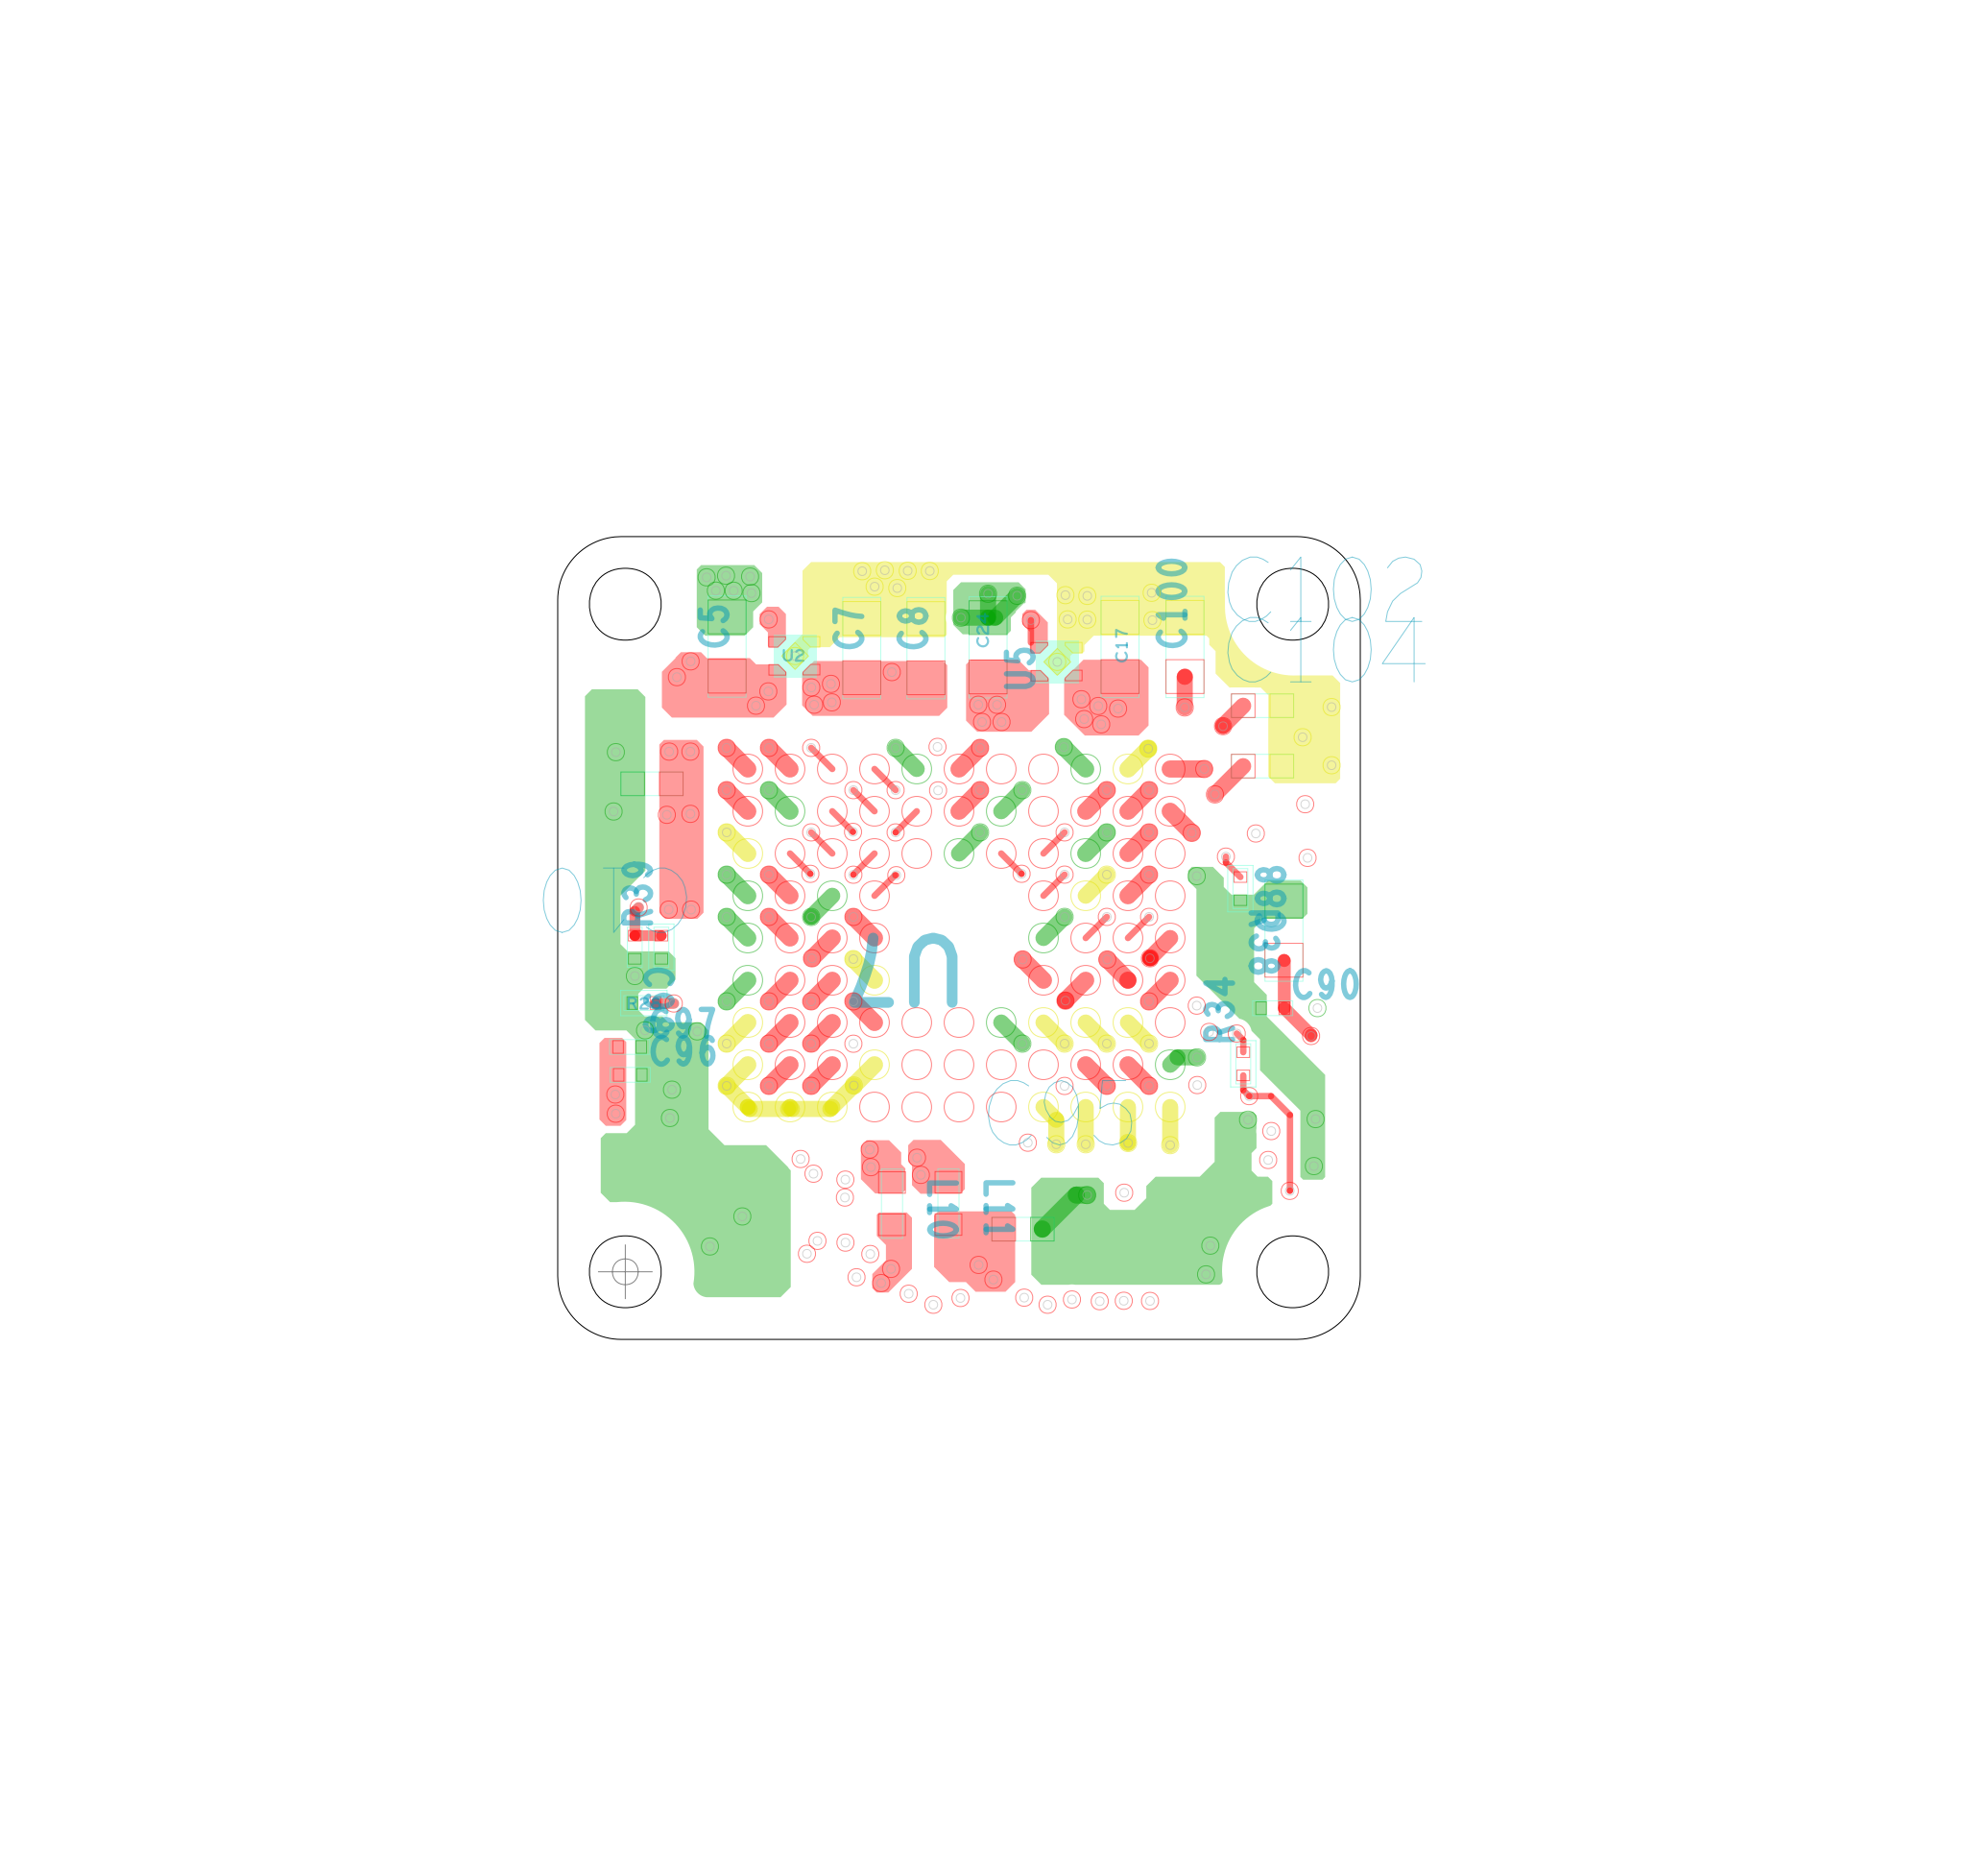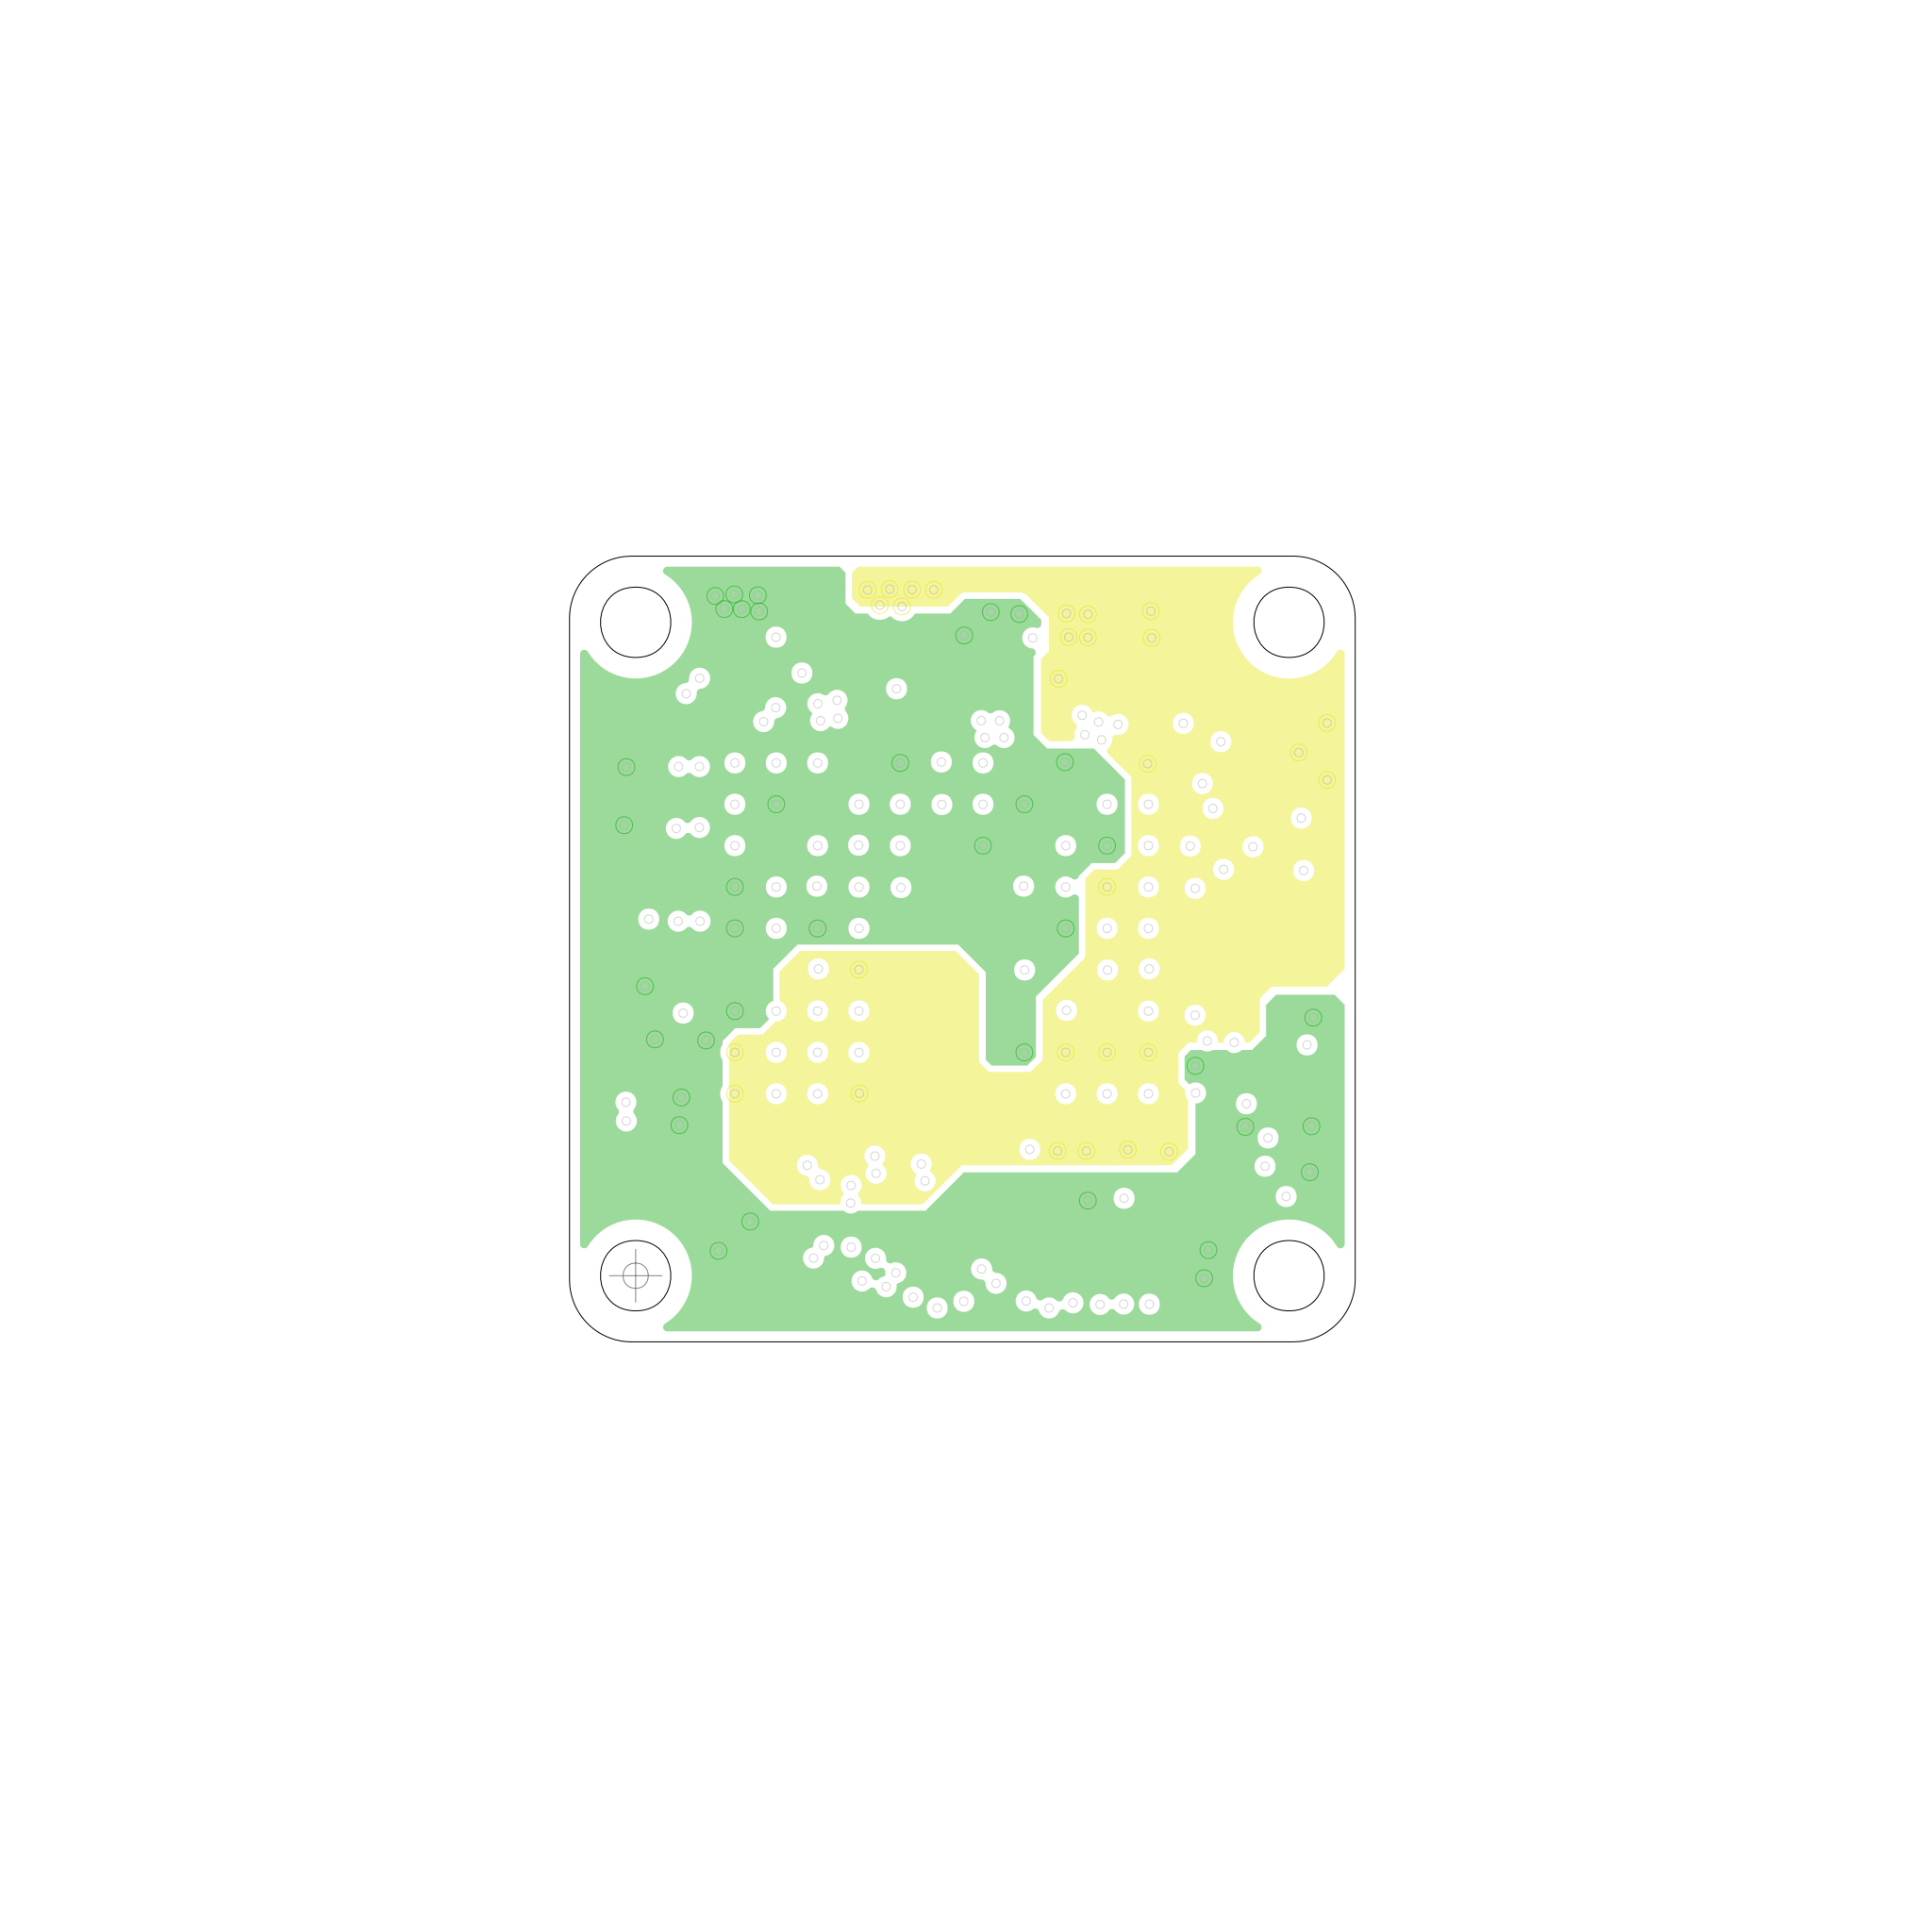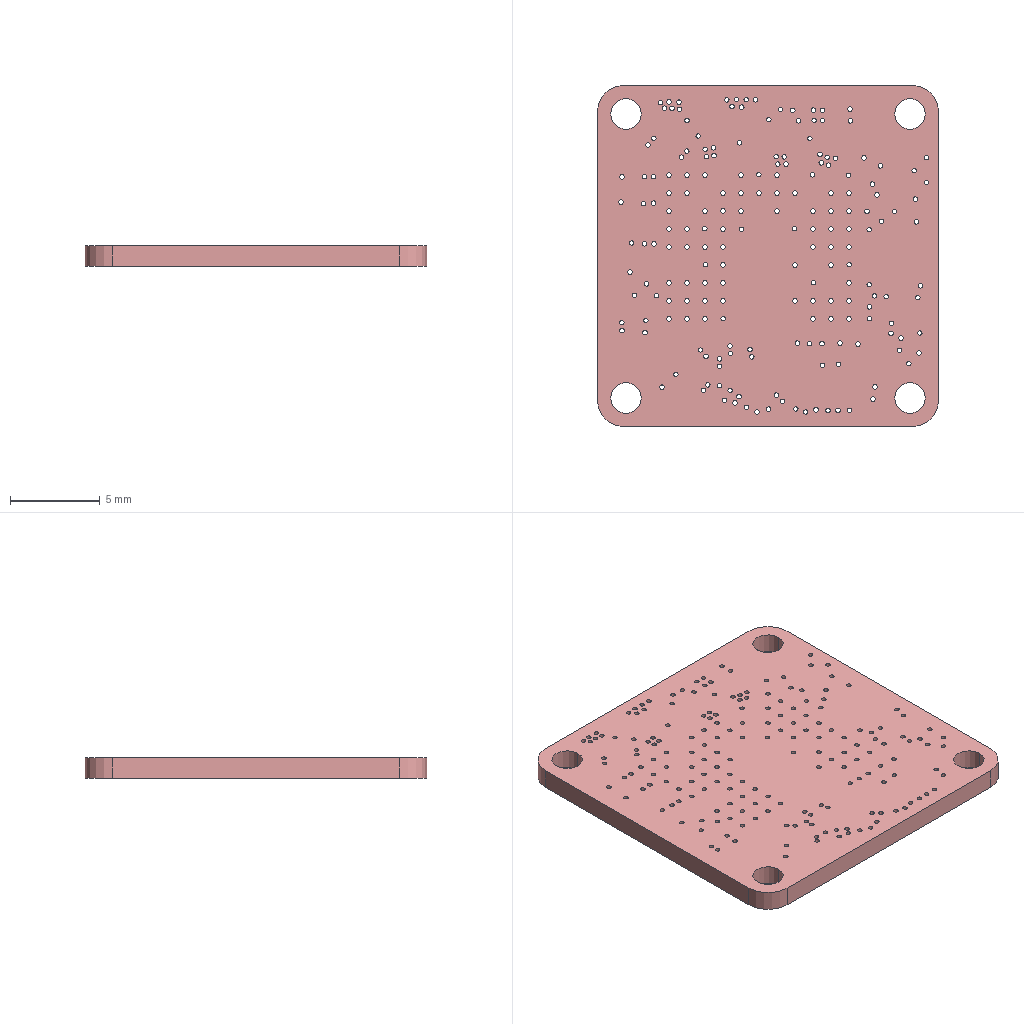Circuit board layout | Cadence Allegro | box 19 x 19 x 1.1 mm
Layer stack:
# Cadence Allegro layer stack of  (unit mm; from the constraint file cross-section; dielectric type: 0 not recorded (Allegro does not mark core vs prepreg), 3 surface material)
index,name,kind,layer,copper_thickness_mm,dielectric_type,dielectric_thickness_mm,dielectric_material,dielectric_constant
0,Top Surface,other,,,,,,
1,TOP,copper,TOP,0.0305,,,,
2,Dielectric1,dielectric,,,0,0.2032,FR-4,4.5
3,GND02,copper,GND02,0.0305,,,,
4,Dielectric2,dielectric,,,0,0.2032,FR-4,4.5
5,SIG03,copper,SIG03,0.0305,,,,
6,Dielectric3,dielectric,,,0,0.2032,FR-4,4.5
7,PWR04,copper,PWR04,0.0305,,,,
8,Dielectric4,dielectric,,,0,0.2032,FR-4,4.5
9,POWER5,copper,POWER5,0.0305,,,,
10,Dielectric5,dielectric,,,0,0.2032,FR-4,4.5
11,BOTTOM,copper,BOTTOM,0.0305,,,,
12,Bottom Surface,other,,,,,,
# drill layer pairs: low layer,high layer
drill_pair,TOP,BOTTOM
Part placement:
REFDES,COMP_VALUE,SYM_NAME,SYM_X,SYM_Y,SYM_ROTATE,SYM_MIRROR
C5,22uF,C0603,94.89,582.62,90.000,NO
C7,22uF,C0603,220.41,581.18,90.000,NO
C8,10uF,C0603,280.21,581.08,90.000,NO
C9,22uF,C0603,19.28,513.11,0.000,YES
C10,10uF,C0402,24.68,454.69,180.000,NO
C11,0.1uF,C0201,153.59,461.18,90.000,YES
C17,22uF,C0603,461.12,582.21,90.000,NO
C18,10uF,C0603,461.58,582.19,270.000,YES
C19,4.7uF,C0402,129.21,412.53,135.000,YES
C20,0.1uF,C0201,114.20,232.60,0.000,YES
C21,0.1uF,C0201,114.42,193.91,0.000,YES
C24,22uF,C0603,338.10,581.90,90.000,NO
C25,22uF,C0603,17.11,198.08,180.000,YES
C28,0.1uF,C0201,389.89,260.78,90.000,YES
C29,0.1uF,C0201,428.89,242.68,90.000,YES
C30,0.1uF,C0201,191.87,270.53,225.000,YES
C80,22uF,C0603,18.79,454.24,0.000,YES
C83,0.1uF,C0201,113.59,310.80,0.000,YES
C84,0.1uF,C0201,194.09,349.40,0.000,YES
C85,4.7uF,C0402,220.47,591.01,270.000,YES
C86,2.2uF,C0201,600.20,192.90,90.000,YES
C87,0.1uF,C0201,348.90,208.99,270.000,YES
C88,22uF,C0603,613.90,317.90,90.000,NO
C89,0.1uF,C0201,509.50,218.20,90.000,YES
C90,2.2uF,C0201,603.40,245.60,0.000,NO
C91,4.7uF,C0402,331.27,574.61,270.000,YES
C92,0.1uF,C0201,364.60,568.20,270.000,YES
C93,4.7uF,C0402,94.47,590.71,270.000,YES
C94,0.1uF,C0201,129.40,572.90,270.000,YES
C95,4.7uF,C0402,370.90,39.70,0.000,NO
C96,2.2uF,C0201,4.60,183.50,0.000,NO
C97,2.2uF,C0201,4.10,209.50,0.000,NO
C98,2.2uF,C0201,8.80,302.39,270.000,NO
C99,22uF,C0603,604.00,527.70,180.000,YES
C100,22uF,C0603,521.66,582.21,90.000,NO
C101,22uF,C0603,603.81,469.66,180.000,YES
C102,4.7uF,C0402,594.11,527.47,0.000,NO
C103,4.7uF,C0402,521.27,573.31,270.000,YES
C104,4.7uF,C0402,594.11,471.17,0.000,NO
J2,MIPI_OUT,J30-0_6MM,122.05,143.31,180.000,YES
L7,4.7uH,IND2-2R0X1R6,-13.58,383.84,180.000,YES
L10,0R,R0402,248.60,63.50,270.000,NO
L11,0R,R0402,301.20,63.70,270.000,NO
L12,NC,R0402,279.90,553.80,90.000,YES
L13,0R,R0402,156.20,635.90,180.000,YES
R27,100K,R0201,63.41,260.82,270.000,YES
R28,115K,R0201,17.32,250.41,0.000,NO
R33,0R,R0201,624.30,193.30,90.000,YES
R34,NC,R0201,576.00,193.80,90.000,NO
R35,1K,R0201,373.51,418.43,180.000,YES
R36,1K,R0201,373.71,392.33,180.000,YES
R37,2K,R0201,553.10,193.90,90.000,YES
R38,0R,R0201,573.30,357.00,270.000,NO
R39,NC,R0201,33.60,302.41,90.000,NO
R40,NC,R0201,609.30,411.10,270.000,YES
R41,NC,R0201,633.70,410.90,270.000,YES
R42,0R,R0201,576.00,193.40,270.000,YES
TP4,TestPoint,TP_0R50,114.82,4.21,0.000,YES
TP6,TestPoint,TP_0R50,155.89,2.37,0.000,YES
TP7,TestPoint,TP_0R50,197.19,-0.23,0.000,YES
TP8,TestPoint,TP_0R50,241.30,204.40,0.000,YES
TP9,TestPoint,TP_0R50,279.40,204.00,0.000,YES
TP10,TestPoint,TP_0R50,78.89,3.97,0.000,YES
U2,SGM2036-1.8V UTDFN,UTDFN_1X1-4L,158.26,573.78,90.000,NO
U5,SGM2036-2.8V UTDFN,UTDFN_1X1-4L,402.63,568.31,90.000,NO
U7,IMX600,SENSOR,311.02,311.02,180.000,NO
U9,MP1601,SOT563_1R5X1R2,28.60,253.90,0.000,YES
U13,MPU6600 QFN24,MCU_QFN20_S120,649.14,343.35,0.000,YES
U14,CZ,0201_3,464.60,4.50,0.000,YES
U15,CZ,0201_3,393.60,5.10,0.000,YES
U16,CZ,0201_3,287.10,5.20,180.000,YES
Pad and via stacks:
# Allegro (Cadence) via spans and padstacks; design units: ("mils" 2 100)
# via spans: padstack,start_layer,end_layer,net_example,count
VIA-8X16,ETCH/TOP,ETCH/BOTTOM,GND,191
# Allegro padstack definitions: name,start_layer,end_layer,drill,plating,holeType,type
S_R0R80X0R90,"ETCH/TOP","ETCH/TOP",0.0,"PLATED","none","smd"
S_R0R25X0R30,"ETCH/TOP","ETCH/TOP",0.0,"NON_PLATED","none","smd"
SMD22_22,"ETCH/TOP","ETCH/TOP",0.0,"PLATED","none","smd"
SMD0D25X0D65,"ETCH/TOP","ETCH/TOP",0.0,"PLATED","none","smd"
SMD0R775_1R0,"ETCH/TOP","ETCH/TOP",0.0,"PLATED","none","smd"
SMD0R7SQ,"ETCH/TOP","ETCH/TOP",0.0,"PLATED","none","smd"
S_R0R70X2R00,"ETCH/TOP","ETCH/TOP",0.0,"NON_PLATED","none","smd"
SMD19_20PSH_L,"ETCH/TOP","ETCH/TOP",0.0,"PLATED","none","smd"
SMD19_20PSH_R,"ETCH/TOP","ETCH/TOP",0.0,"PLATED","none","smd"
SMD_BOTTOM_R350X300P0S40,"ETCH/TOP","ETCH/TOP",0.0,"PLATED","none","smd"
S_C0R50,"ETCH/TOP","ETCH/TOP",0.0,"NON_PLATED","none","smd"
SMD40REC20,"ETCH/TOP","ETCH/TOP",0.0,"PLATED","none","smd"
S_S0R45,"ETCH/TOP","ETCH/TOP",0.0,"NON_PLATED","none","smd"
UTDFN_1,"ETCH/TOP","ETCH/TOP",0.0,"PLATED","none","smd"
UTDFN_2,"ETCH/TOP","ETCH/TOP",0.0,"PLATED","none","smd"
SMD5-0,"ETCH/TOP","ETCH/TOP",0.0,"NON_PLATED","none","smd"
SMD0-8_0-15,"ETCH/TOP","ETCH/TOP",0.0,"NON_PLATED","none","smd"
SMD_C118P0S40,"ETCH/TOP","ETCH/TOP",0.0,"PLATED","none","smd"
SMD_R12X27,"ETCH/TOP","ETCH/TOP",0.0,"PLATED","none","smd"
SMD_R118X236P0S40,"ETCH/TOP","ETCH/TOP",0.0,"PLATED","none","smd"
SMD_0D8X0D9,"ETCH/TOP","ETCH/TOP",0.0,"PLATED","none","smd"
SMD5-0-1,"ETCH/TOP","ETCH/TOP",0.0,"NON_PLATED","none","smd"
SMD59_35,"ETCH/TOP","ETCH/TOP",0.0,"PLATED","none","smd"
P_C0R40_C0R65,"ETCH/TOP","ETCH/BOTTOM",15.7,"PLATED","circle_drill","through"
VIA,"ETCH/TOP","ETCH/BOTTOM",13.0,"PLATED","circle_drill","through"
VIA_FORPCB_8X16,"ETCH/TOP","ETCH/BOTTOM",8.0,"PLATED","circle_drill","through"
PTH_C1063D984S50,"ETCH/TOP","ETCH/BOTTOM",74.8,"PLATED","circle_drill","through"
HOLE2-3_5,"ETCH/TOP","ETCH/BOTTOM",82.7,"PLATED","circle_drill","through"
VIA_FORPCB_10X18,"ETCH/TOP","ETCH/BOTTOM",10.0,"PLATED","circle_drill","through"
SMD0R45_CIR,"ETCH/TOP","ETCH/TOP",0.0,"PLATED","none","smd"
SMD1R1_SQ,"ETCH/TOP","ETCH/TOP",0.0,"PLATED","none","smd"
S_C0R50-1,"ETCH/TOP","ETCH/TOP",0.0,"NON_PLATED","none","smd"
S_C0R50-2,"ETCH/TOP","ETCH/TOP",0.0,"NON_PLATED","none","smd"
SMD1R0_CIR,"ETCH/TOP","ETCH/TOP",0.0,"PLATED","none","smd"
SMD1R6X0R7,"ETCH/TOP","ETCH/TOP",0.0,"PLATED","none","smd"
SMD0-25_0-7OB,"ETCH/TOP","ETCH/TOP",0.0,"NON_PLATED","none","smd"
SMD1-25_0-675,"ETCH/TOP","ETCH/TOP",0.0,"PLATED","none","smd"
RECT20X25,"ETCH/TOP","ETCH/TOP",0.0,"PLATED","none","smd"
SMD_C276P0S40,"ETCH/TOP","ETCH/TOP",0.0,"PLATED","none","smd"
SMD_R79X197P0S10,"ETCH/TOP","ETCH/TOP",0.0,"PLATED","none","smd"
SMD_S276P0S10,"ETCH/TOP","ETCH/TOP",0.0,"PLATED","none","smd"
SMD_R472X276P0S10,"ETCH/TOP","ETCH/TOP",0.0,"PLATED","none","smd"
SMD_R394X276P0S10,"ETCH/TOP","ETCH/TOP",0.0,"PLATED","none","smd"
SMD_R79X110P0S10,"ETCH/TOP","ETCH/TOP",0.0,"PLATED","none","smd"
SMD_O236X87P0S10,"ETCH/TOP","ETCH/TOP",0.0,"PLATED","none","smd"
SMD_R669X630P0S10,"ETCH/TOP","ETCH/TOP",0.0,"PLATED","none","smd"
VIA-8X16,"ETCH/TOP","ETCH/BOTTOM",8.0,"PLATED","circle_drill","through"
Design rules, without the lines most boards share, first 14 of 26 lines:
# Cadence Allegro design rules of  (from the Constraint Manager export constraints.dcfx, design unit mil; typed fields in mm)
# columns: name | kind | enabled | priority | scope1 | scope2 | descriptor | typed fields (field=value)
# Allegro precedence (priority 1 wins): 1 Region class-to-class, 2 Region class, 3 Region, 4 class-to-class, 5 DiffPair/Bus/NetGroup override, 6 NetClass, 7 constraint set (CSet) default
# per-layer values are written LAYER=value in the descriptor and LAYER:mm in the typed field; a maximum of 0 means no limit set
# --- net classes (and buses / net groups) ---
U13_CLASS | NetClass | enabled | 6 | D2P-2A, D2N-2B, 2C | All | Net Class (members: 3 Xnet) |
U15_CLASS | NetClass | enabled | 6 | D1N-1A, CKP-1B, CKN-1C | All | Net Class (members: 3 Xnet) |
U14_CLASS | NetClass | enabled | 6 | D3P-0A, D3N-0B, D1P-0C | All | Net Class (members: 3 Xnet) |
# --- track widths, neck and differential-pair gap (physical constraint sets) ---
DEFAULT | PhysicalCSet | enabled | 7 | Design default | All | Physical Constraint (Min Line Width=6mil) (Max Line Width=40mil) (Min Neck Width=6mil) (Max Neck Length=0mil) (DiffPair Primary Gap=6mil) (DiffPair Neck Gap=0mil) (DiffPair Min Space=6mil) (DiffPair Coupled +Tol=0mil) (DiffPair Coupled -Tol=0mil) (Min BB Via Stagger=6mil) (Max BB Via Stagger=0mil) (T-junctions=ANYWHERE) (Pad-pad direct connect=ALL_ALLOWED) (Allowed vias=VIA-8X16) | min_line_width=0.1524 min_neck_width=0.1524 min_bvia_stagger=0.1524 max_bvia_stagger=0 ts_allowed=ANYWHERE diffp_primary_gap=0.1524 diffp_neck_gap=0 max_line_width=1.016 maximum_neck_length=0 pad_pad_direct_connect=ALL_ALLOWED allow_on_etch_subclass=TRUE diffp_coupled_plus=0 diffp_coupled_minus=0 diffp_min_space=0.1524 vias=VIA-8X16
# --- clearances: line / pad / via / shape / hole (spacing constraint sets) ---
DEFAULT | SpacingCSet | enabled | 7 | Design default | All | Clearance Constraint (Line-Line=6mil) (Line-SMD Pad=6mil) (Line-Thru Pin=6mil) (Line-Via=6mil) (Line-Shape=6mil) (SMD Pad-SMD Pad=TOP=5mil GND02=6mil SIG03=5mil PWR04=6mil POWER5=6mil BOTTOM=5mil) (Thru Pin-Thru Pin=6mil) (Thru Pin-SMD Pad=6mil) (SMD Pad-Via=6mil) (Thru Pin-Via=6mil) (Via-Via=6mil) (Shape-SMD Pad=6mil) (Shape-Thru Pin=6mil) (Shape-Via=6mil) (Shape-Shape=6mil) (Hole-Hole=6mil) (Hole-Line=6mil) (Hole-Shape=6mil) (BB Via-BB Via=6mil) (uVia-uVia=4mil) | thrupin_to_thrupin_spacing=0.1524 thrupin_to_smdpin_spacing=0.1524 thrupin_to_thruvia_spacing=0.1524 line_to_thrupin_spacing=0.1524 thrupin_to_shape_spacing=0.1524 smdpin_to_smdpin_spacing=TOP:0.127,GND02:0.1524,SIG03:0.127,PWR04:0.1524,POWER5:0.1524,BOTTOM:0.127 smdpin_to_thruvia_spacing=0.1524 line_to_smdpin_spacing=0.1524 shape_to_smdpin_spacing=0.1524 thruvia_to_thruvia_spacing=0.1524 line_to_thruvia_spacing=0.1524 shape_to_thruvia_spacing=0.1524 line_to_line_spacing=0.1524 line_to_shape_spacing=0.1524 shape_to_shape_spacing=0.1524 bbv_to_bbv_spacing=0.1524 bbv_to_thrupin_spacing=0.1524 bbv_to_smdpin_spacing=0.1524 bbv_to_thruvia_spacing=0.1524 bbv_to_line_spacing=0.1524 bbv_to_shape_spacing=0.1524 bbv_to_testpin_spacing=0.1524 bbv_to_testvia_spacing=0.1524 testpin_to_testpin_spacing=0.1524 testpin_to_thrupin_spacing=0.1524 smdpin_to_testpin_spacing=0.1524 testpin_to_thruvia_spacing=0.1524 testpin_to_testvia_spacing=0.1524 line_to_testpin_spacing=0.1524 shape_to_testpin_spacing=0.1524 testvia_to_testvia_spacing=0.1524 testvia_to_thrupin_spacing=0.1524 smdpin_to_testvia_spacing=0.1524 testvia_to_thruvia_spacing=0.1524 line_to_testvia_spacing=0.1524 shape_to_testvia_spacing=0.1524 bondpad_to_bondpad_spacing=0.1524 thrupin_to_bondpad_spacing=0.1524 smdpin_to_bondpad_spacing=0.1524 bondpad_to_thruvia_spacing=0.1524 bondpad_to_line_spacing=0.1524 bondpad_to_shape_spacing=0.1524 bondpad_to_bbv_spacing=0.1524 bondpad_to_testpin_spacing=0.1524 bondpad_to_testvia_spacing=0.1524 min_bvia_gap=0.1524 hole_to_pin_spacing=0.1524 hole_to_via_spacing=0.1524 hole_to_line_spacing=0.1524 hole_to_shape_spacing=0.1524 hole_to_hole_spacing=0.1524 mvia_to_mvia_spacing=0.1016 mvia_to_thrupin_spacing=0.1016 mvia_to_smdpin_spacing=0.1016 mvia_to_thruvia_spacing=0.1016 mvia_to_bbv_spacing=0.1016 mvia_to_line_spacing=0.1016 mvia_to_shape_spacing=0.1524 mvia_to_testpin_spacing=0.1016 mvia_to_testvia_spacing=0.1016 bondpad_to_mvia_spacing=0.1016 bondpad_to_bondpad_diffp_spc=0.127
DEFAULT | SameNetSpacingCSet | enabled | 7 | Design default | All | Same-Net Clearance (Line-Line=5mil) (Line-SMD Pad=5mil) (Line-Thru Pin=5mil) (Line-Via=5mil) (Line-Shape=5mil) (SMD Pad-SMD Pad=5mil) (Thru Pin-Thru Pin=5mil) (Thru Pin-SMD Pad=5mil) (SMD Pad-Via=5mil) (Thru Pin-Via=5mil) (Via-Via=5mil) (Shape-SMD Pad=5mil) (Shape-Thru Pin=5mil) (Shape-Via=5mil) (Shape-Shape=5mil) (Hole-Hole=8mil) (Hole-Line=8mil) (Hole-Shape=8mil) (BB Via-BB Via=5mil) (uVia-uVia=5mil) | sn_thrupin_to_thrupin_spacing=0.127 sn_thrupin_to_smdpin_spacing=0.127 sn_thrupin_to_thruvia_spacing=0.127 sn_line_to_thrupin_spacing=0.127 sn_thrupin_to_shape_spacing=0.127 sn_smdpin_to_smdpin_spacing=0.127 sn_smdpin_to_thruvia_spacing=0.127 sn_line_to_smdpin_spacing=0.127 sn_shape_to_smdpin_spacing=0.127 sn_thruvia_to_thruvia_spacing=0.127 sn_line_to_thruvia_spacing=0.127 sn_shape_to_thruvia_spacing=0.127 sn_line_to_line_spacing=0.127 sn_line_to_shape_spacing=0.127 sn_shape_to_shape_spacing=0.127 sn_bbv_to_bbv_spacing=0.127 sn_bbv_to_thrupin_spacing=0.127 sn_bbv_to_smdpin_spacing=0.127 sn_bbv_to_thruvia_spacing=0.127 sn_bbv_to_line_spacing=0.127 sn_bbv_to_shape_spacing=0.127 sn_bbv_to_testpin_spacing=0.127 sn_bbv_to_testvia_spacing=0.127 sn_testpin_to_testpin_spacing=0.127 sn_testpin_to_thrupin_spacing=0.127 sn_smdpin_to_testpin_spacing=0.127 sn_testpin_to_thruvia_spacing=0.127 sn_testpin_to_testvia_spacing=0.127 sn_line_to_testpin_spacing=0.127 sn_shape_to_testpin_spacing=0.127 sn_testvia_to_testvia_spacing=0.127 sn_testvia_to_thrupin_spacing=0.127 sn_smdpin_to_testvia_spacing=0.127 sn_testvia_to_thruvia_spacing=0.127 sn_line_to_testvia_spacing=0.127 sn_shape_to_testvia_spacing=0.127 sn_bondpad_to_bondpad_spacing=0.127 sn_thrupin_to_bondpad_spacing=0.127 sn_smdpin_to_bondpad_spacing=0.127 sn_bondpad_to_thruvia_spacing=0.127 sn_bondpad_to_line_spacing=0.127 sn_bondpad_to_shape_spacing=0.127 sn_bondpad_to_bbv_spacing=0.127 sn_bondpad_to_testpin_spacing=0.127 sn_bondpad_to_testvia_spacing=0.127 same_net=TRUE sn_hole_to_pin_spacing=0.2032 sn_hole_to_via_spacing=0.2032 sn_hole_to_line_spacing=0.2032 sn_hole_to_shape_spacing=0.2032 sn_hole_to_hole_spacing=0.2032 sn_mvia_to_mvia_spacing=0.127 sn_mvia_to_thrupin_spacing=0.127 sn_mvia_to_smdpin_spacing=0.127 sn_mvia_to_thruvia_spacing=0.127 sn_mvia_to_bbv_spacing=0.127 sn_mvia_to_line_spacing=0.127 sn_mvia_to_shape_spacing=0.127 sn_mvia_to_testpin_spacing=0.127 sn_mvia_to_testvia_spacing=0.127 sn_bondpad_to_mvia_spacing=0.127
# --- differential pairs (0) ---